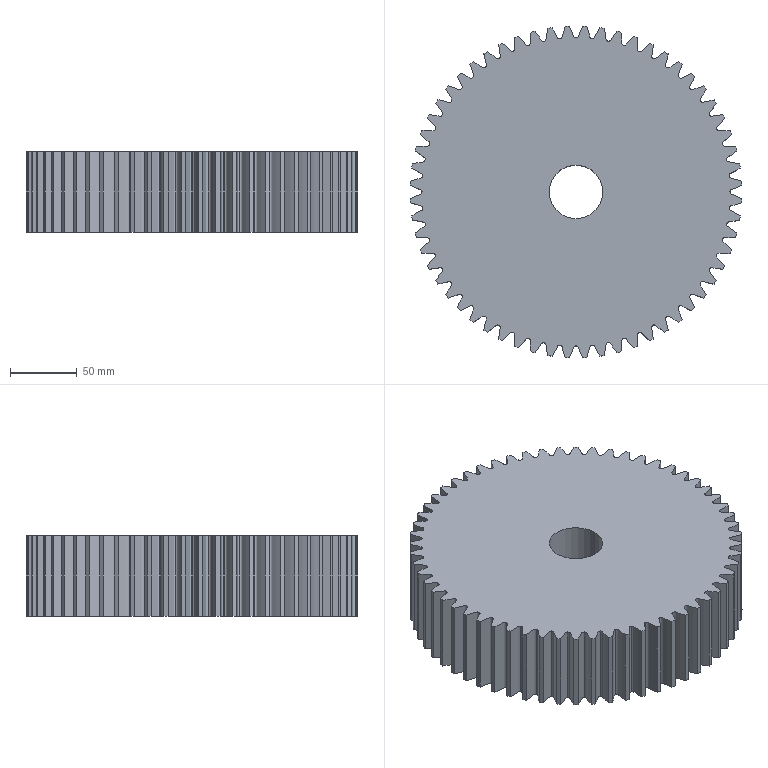Part | SolidWorks | features BaseBody 1 | 1 solid | 245 faces | box 247.805 x 247.805 x 60 mm | volume 2631200 mm3 | cylinder 123 | spline 120 | plane 2 | commonest cylinder face diameters 230 x61 248 x60 40 x2